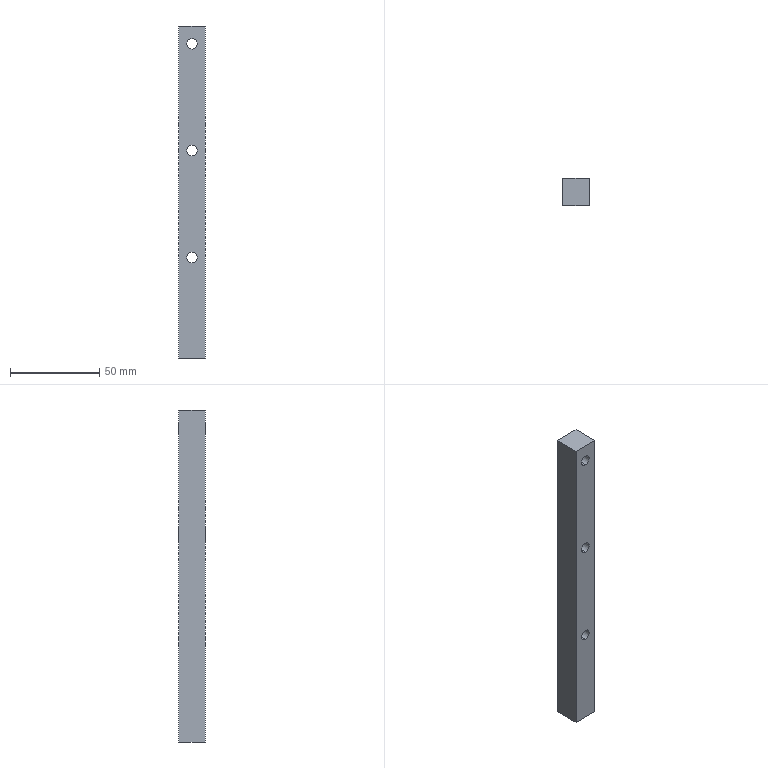Part | 1 solid | 16 faces | box 15 x 15 x 186.5 mm | volume 40084 mm3 | cylinder 8 | plane 6 | cone 2 | commonest cylinder face diameters 6 x6 6.8 x2
STEP:
#1=CARTESIAN_POINT('',(10.9,7.5,89.5));
#2=VERTEX_POINT('',#1);
#3=CARTESIAN_POINT('',(4.1,7.5,89.5));
#4=VERTEX_POINT('',#3);
#5=CARTESIAN_POINT('',(7.5,7.5,89.5));
#6=DIRECTION('',(0.,0.,-1.));
#7=DIRECTION('',(-1.,0.,0.));
#8=AXIS2_PLACEMENT_3D('',#5,#6,#7);
#9=CIRCLE('',#8,3.4);
#10=EDGE_CURVE('',#2,#4,#9,.T.);
#11=ORIENTED_EDGE('',*,*,#10,.F.);
#12=CARTESIAN_POINT('',(10.9,7.5,73.5));
#13=VERTEX_POINT('',#12);
#14=CARTESIAN_POINT('',(10.9,7.5,73.5));
#15=DIRECTION('',(0.,0.,-1.));
#16=VECTOR('',#15,1000.);
#17=LINE('',#14,#16);
#18=EDGE_CURVE('',#2,#13,#17,.T.);
#19=ORIENTED_EDGE('',*,*,#18,.T.);
#20=CARTESIAN_POINT('',(4.1,7.5,73.5));
#21=VERTEX_POINT('',#20);
#22=CARTESIAN_POINT('',(7.5,7.5,73.5));
#23=DIRECTION('',(0.,0.,-1.));
#24=DIRECTION('',(-1.,0.,0.));
#25=AXIS2_PLACEMENT_3D('',#22,#23,#24);
#26=CIRCLE('',#25,3.4);
#27=EDGE_CURVE('',#13,#21,#26,.T.);
#28=ORIENTED_EDGE('',*,*,#27,.T.);
#29=CARTESIAN_POINT('',(4.1,7.5,73.5));
#30=DIRECTION('',(0.,0.,-1.));
#31=VECTOR('',#30,1000.);
#32=LINE('',#29,#31);
#33=EDGE_CURVE('',#4,#21,#32,.T.);
#34=ORIENTED_EDGE('',*,*,#33,.F.);
#35=EDGE_LOOP('',(#11,#19,#28,#34));
#36=FACE_OUTER_BOUND('',#35,.T.);
#37=CARTESIAN_POINT('',(7.5,7.5,73.5));
#38=DIRECTION('',(0.,0.,-1.));
#39=DIRECTION('',(-1.,0.,0.));
#40=AXIS2_PLACEMENT_3D('',#37,#38,#39);
#41=CYLINDRICAL_SURFACE('',#40,3.4);
#42=ADVANCED_FACE('',(#36),#41,.F.);
#43=CARTESIAN_POINT('',(7.5,7.5,91.543));
#44=VERTEX_POINT('',#43);
#45=CARTESIAN_POINT('',(4.1,7.5,89.5));
#46=DIRECTION('',(-0.8572,0.,-0.515));
#47=VECTOR('',#46,1000.);
#48=LINE('',#45,#47);
#49=EDGE_CURVE('',#44,#4,#48,.T.);
#50=ORIENTED_EDGE('',*,*,#49,.F.);
#51=CARTESIAN_POINT('',(10.9,7.5,89.5));
#52=DIRECTION('',(0.8572,0.,-0.515));
#53=VECTOR('',#52,1000.);
#54=LINE('',#51,#53);
#55=EDGE_CURVE('',#44,#2,#54,.T.);
#56=ORIENTED_EDGE('',*,*,#55,.T.);
#57=ORIENTED_EDGE('',*,*,#10,.T.);
#58=EDGE_LOOP('',(#50,#56,#57));
#59=FACE_OUTER_BOUND('',#58,.T.);
#60=CARTESIAN_POINT('',(7.5,7.5,89.5));
#61=DIRECTION('',(0.,0.,-1.));
#62=DIRECTION('',(-1.,0.,0.));
#63=AXIS2_PLACEMENT_3D('',#60,#61,#62);
#64=CONICAL_SURFACE('',#63,3.4,1.03);
#65=ADVANCED_FACE('',(#59),#64,.F.);
#66=CARTESIAN_POINT('',(7.5,0.,247.));
#67=VERTEX_POINT('',#66);
#68=CARTESIAN_POINT('',(7.5,0.,253.));
#69=VERTEX_POINT('',#68);
#70=CARTESIAN_POINT('',(7.5,0.,250.));
#71=DIRECTION('',(0.,1.,0.));
#72=DIRECTION('',(0.,0.,1.));
#73=AXIS2_PLACEMENT_3D('',#70,#71,#72);
#74=CIRCLE('',#73,3.);
#75=EDGE_CURVE('',#67,#69,#74,.T.);
#76=ORIENTED_EDGE('',*,*,#75,.F.);
#77=CARTESIAN_POINT('',(7.5,15.,247.));
#78=VERTEX_POINT('',#77);
#79=CARTESIAN_POINT('',(7.5,-35.,247.));
#80=DIRECTION('',(0.,1.,0.));
#81=VECTOR('',#80,1000.);
#82=LINE('',#79,#81);
#83=EDGE_CURVE('',#67,#78,#82,.T.);
#84=ORIENTED_EDGE('',*,*,#83,.T.);
#85=CARTESIAN_POINT('',(7.5,15.,253.));
#86=VERTEX_POINT('',#85);
#87=CARTESIAN_POINT('',(7.5,15.,250.));
#88=DIRECTION('',(0.,1.,0.));
#89=DIRECTION('',(0.,0.,1.));
#90=AXIS2_PLACEMENT_3D('',#87,#88,#89);
#91=CIRCLE('',#90,3.);
#92=EDGE_CURVE('',#78,#86,#91,.T.);
#93=ORIENTED_EDGE('',*,*,#92,.T.);
#94=CARTESIAN_POINT('',(7.5,-35.,253.));
#95=DIRECTION('',(0.,1.,0.));
#96=VECTOR('',#95,1000.);
#97=LINE('',#94,#96);
#98=EDGE_CURVE('',#69,#86,#97,.T.);
#99=ORIENTED_EDGE('',*,*,#98,.F.);
#100=EDGE_LOOP('',(#76,#84,#93,#99));
#101=FACE_OUTER_BOUND('',#100,.T.);
#102=CARTESIAN_POINT('',(7.5,-35.,250.));
#103=DIRECTION('',(0.,1.,0.));
#104=DIRECTION('',(0.,0.,1.));
#105=AXIS2_PLACEMENT_3D('',#102,#103,#104);
#106=CYLINDRICAL_SURFACE('',#105,3.);
#107=ADVANCED_FACE('',(#101),#106,.F.);
#108=CARTESIAN_POINT('',(7.5,0.,187.));
#109=VERTEX_POINT('',#108);
#110=CARTESIAN_POINT('',(7.5,0.,193.));
#111=VERTEX_POINT('',#110);
#112=CARTESIAN_POINT('',(7.5,0.,190.));
#113=DIRECTION('',(0.,1.,0.));
#114=DIRECTION('',(0.,0.,1.));
#115=AXIS2_PLACEMENT_3D('',#112,#113,#114);
#116=CIRCLE('',#115,3.);
#117=EDGE_CURVE('',#109,#111,#116,.T.);
#118=ORIENTED_EDGE('',*,*,#117,.F.);
#119=CARTESIAN_POINT('',(7.5,15.,187.));
#120=VERTEX_POINT('',#119);
#121=CARTESIAN_POINT('',(7.5,-35.,187.));
#122=DIRECTION('',(0.,1.,0.));
#123=VECTOR('',#122,1000.);
#124=LINE('',#121,#123);
#125=EDGE_CURVE('',#109,#120,#124,.T.);
#126=ORIENTED_EDGE('',*,*,#125,.T.);
#127=CARTESIAN_POINT('',(7.5,15.,193.));
#128=VERTEX_POINT('',#127);
#129=CARTESIAN_POINT('',(7.5,15.,190.));
#130=DIRECTION('',(0.,1.,0.));
#131=DIRECTION('',(0.,0.,1.));
#132=AXIS2_PLACEMENT_3D('',#129,#130,#131);
#133=CIRCLE('',#132,3.);
#134=EDGE_CURVE('',#120,#128,#133,.T.);
#135=ORIENTED_EDGE('',*,*,#134,.T.);
#136=CARTESIAN_POINT('',(7.5,-35.,193.));
#137=DIRECTION('',(0.,1.,0.));
#138=VECTOR('',#137,1000.);
#139=LINE('',#136,#138);
#140=EDGE_CURVE('',#111,#128,#139,.T.);
#141=ORIENTED_EDGE('',*,*,#140,.F.);
#142=EDGE_LOOP('',(#118,#126,#135,#141));
#143=FACE_OUTER_BOUND('',#142,.T.);
#144=CARTESIAN_POINT('',(7.5,-35.,190.));
#145=DIRECTION('',(0.,1.,0.));
#146=DIRECTION('',(0.,0.,1.));
#147=AXIS2_PLACEMENT_3D('',#144,#145,#146);
#148=CYLINDRICAL_SURFACE('',#147,3.);
#149=ADVANCED_FACE('',(#143),#148,.F.);
#150=CARTESIAN_POINT('',(7.5,0.,127.));
#151=VERTEX_POINT('',#150);
#152=CARTESIAN_POINT('',(7.5,0.,133.));
#153=VERTEX_POINT('',#152);
#154=CARTESIAN_POINT('',(7.5,0.,130.));
#155=DIRECTION('',(0.,1.,0.));
#156=DIRECTION('',(0.,0.,1.));
#157=AXIS2_PLACEMENT_3D('',#154,#155,#156);
#158=CIRCLE('',#157,3.);
#159=EDGE_CURVE('',#151,#153,#158,.T.);
#160=ORIENTED_EDGE('',*,*,#159,.F.);
#161=CARTESIAN_POINT('',(7.5,15.,127.));
#162=VERTEX_POINT('',#161);
#163=CARTESIAN_POINT('',(7.5,-35.,127.));
#164=DIRECTION('',(0.,1.,0.));
#165=VECTOR('',#164,1000.);
#166=LINE('',#163,#165);
#167=EDGE_CURVE('',#151,#162,#166,.T.);
#168=ORIENTED_EDGE('',*,*,#167,.T.);
#169=CARTESIAN_POINT('',(7.5,15.,133.));
#170=VERTEX_POINT('',#169);
#171=CARTESIAN_POINT('',(7.5,15.,130.));
#172=DIRECTION('',(0.,1.,0.));
#173=DIRECTION('',(0.,0.,1.));
#174=AXIS2_PLACEMENT_3D('',#171,#172,#173);
#175=CIRCLE('',#174,3.);
#176=EDGE_CURVE('',#162,#170,#175,.T.);
#177=ORIENTED_EDGE('',*,*,#176,.T.);
#178=CARTESIAN_POINT('',(7.5,-35.,133.));
#179=DIRECTION('',(0.,1.,0.));
#180=VECTOR('',#179,1000.);
#181=LINE('',#178,#180);
#182=EDGE_CURVE('',#153,#170,#181,.T.);
#183=ORIENTED_EDGE('',*,*,#182,.F.);
#184=EDGE_LOOP('',(#160,#168,#177,#183));
#185=FACE_OUTER_BOUND('',#184,.T.);
#186=CARTESIAN_POINT('',(7.5,-35.,130.));
#187=DIRECTION('',(0.,1.,0.));
#188=DIRECTION('',(0.,0.,1.));
#189=AXIS2_PLACEMENT_3D('',#186,#187,#188);
#190=CYLINDRICAL_SURFACE('',#189,3.);
#191=ADVANCED_FACE('',(#185),#190,.F.);
#192=CARTESIAN_POINT('',(0.,0.,73.5));
#193=VERTEX_POINT('',#192);
#194=CARTESIAN_POINT('',(0.,15.,73.5));
#195=VERTEX_POINT('',#194);
#196=CARTESIAN_POINT('',(0.,0.,73.5));
#197=DIRECTION('',(0.,1.,0.));
#198=VECTOR('',#197,1000.);
#199=LINE('',#196,#198);
#200=EDGE_CURVE('',#193,#195,#199,.T.);
#201=ORIENTED_EDGE('',*,*,#200,.F.);
#202=CARTESIAN_POINT('',(0.,0.,260.));
#203=VERTEX_POINT('',#202);
#204=CARTESIAN_POINT('',(0.,0.,700.));
#205=DIRECTION('',(0.,0.,-1.));
#206=VECTOR('',#205,1000.);
#207=LINE('',#204,#206);
#208=EDGE_CURVE('',#203,#193,#207,.T.);
#209=ORIENTED_EDGE('',*,*,#208,.F.);
#210=CARTESIAN_POINT('',(0.,15.,260.));
#211=VERTEX_POINT('',#210);
#212=CARTESIAN_POINT('',(0.,15.,260.));
#213=DIRECTION('',(0.,-1.,0.));
#214=VECTOR('',#213,1000.);
#215=LINE('',#212,#214);
#216=EDGE_CURVE('',#211,#203,#215,.T.);
#217=ORIENTED_EDGE('',*,*,#216,.F.);
#218=CARTESIAN_POINT('',(0.,15.,700.));
#219=DIRECTION('',(0.,0.,-1.));
#220=VECTOR('',#219,1000.);
#221=LINE('',#218,#220);
#222=EDGE_CURVE('',#211,#195,#221,.T.);
#223=ORIENTED_EDGE('',*,*,#222,.T.);
#224=EDGE_LOOP('',(#201,#209,#217,#223));
#225=FACE_OUTER_BOUND('',#224,.T.);
#226=CARTESIAN_POINT('',(0.,0.,700.));
#227=DIRECTION('',(1.,0.,0.));
#228=DIRECTION('',(0.,0.,-1.));
#229=AXIS2_PLACEMENT_3D('',#226,#227,#228);
#230=PLANE('',#229);
#231=ADVANCED_FACE('',(#225),#230,.F.);
#232=CARTESIAN_POINT('',(7.5,0.,130.));
#233=DIRECTION('',(0.,1.,0.));
#234=DIRECTION('',(0.,0.,1.));
#235=AXIS2_PLACEMENT_3D('',#232,#233,#234);
#236=CIRCLE('',#235,3.);
#237=EDGE_CURVE('',#153,#151,#236,.T.);
#238=ORIENTED_EDGE('',*,*,#237,.T.);
#239=ORIENTED_EDGE('',*,*,#159,.T.);
#240=EDGE_LOOP('',(#238,#239));
#241=FACE_BOUND('',#240,.T.);
#242=CARTESIAN_POINT('',(7.5,0.,190.));
#243=DIRECTION('',(0.,1.,0.));
#244=DIRECTION('',(0.,0.,1.));
#245=AXIS2_PLACEMENT_3D('',#242,#243,#244);
#246=CIRCLE('',#245,3.);
#247=EDGE_CURVE('',#111,#109,#246,.T.);
#248=ORIENTED_EDGE('',*,*,#247,.T.);
#249=ORIENTED_EDGE('',*,*,#117,.T.);
#250=EDGE_LOOP('',(#248,#249));
#251=FACE_BOUND('',#250,.T.);
#252=CARTESIAN_POINT('',(7.5,0.,250.));
#253=DIRECTION('',(0.,1.,0.));
#254=DIRECTION('',(0.,0.,1.));
#255=AXIS2_PLACEMENT_3D('',#252,#253,#254);
#256=CIRCLE('',#255,3.);
#257=EDGE_CURVE('',#69,#67,#256,.T.);
#258=ORIENTED_EDGE('',*,*,#257,.T.);
#259=ORIENTED_EDGE('',*,*,#75,.T.);
#260=EDGE_LOOP('',(#258,#259));
#261=FACE_BOUND('',#260,.T.);
#262=CARTESIAN_POINT('',(15.,0.,73.5));
#263=VERTEX_POINT('',#262);
#264=CARTESIAN_POINT('',(15.,0.,73.5));
#265=DIRECTION('',(-1.,0.,0.));
#266=VECTOR('',#265,1000.);
#267=LINE('',#264,#266);
#268=EDGE_CURVE('',#263,#193,#267,.T.);
#269=ORIENTED_EDGE('',*,*,#268,.F.);
#270=CARTESIAN_POINT('',(15.,0.,260.));
#271=VERTEX_POINT('',#270);
#272=CARTESIAN_POINT('',(15.,0.,700.));
#273=DIRECTION('',(0.,0.,-1.));
#274=VECTOR('',#273,1000.);
#275=LINE('',#272,#274);
#276=EDGE_CURVE('',#271,#263,#275,.T.);
#277=ORIENTED_EDGE('',*,*,#276,.F.);
#278=CARTESIAN_POINT('',(0.,0.,260.));
#279=DIRECTION('',(1.,0.,0.));
#280=VECTOR('',#279,1000.);
#281=LINE('',#278,#280);
#282=EDGE_CURVE('',#203,#271,#281,.T.);
#283=ORIENTED_EDGE('',*,*,#282,.F.);
#284=ORIENTED_EDGE('',*,*,#208,.T.);
#285=EDGE_LOOP('',(#269,#277,#283,#284));
#286=FACE_OUTER_BOUND('',#285,.T.);
#287=CARTESIAN_POINT('',(0.,0.,700.));
#288=DIRECTION('',(0.,1.,0.));
#289=DIRECTION('',(0.,0.,1.));
#290=AXIS2_PLACEMENT_3D('',#287,#288,#289);
#291=PLANE('',#290);
#292=ADVANCED_FACE('',(#241,#251,#261,#286),#291,.F.);
#293=CARTESIAN_POINT('',(15.,15.,73.5));
#294=VERTEX_POINT('',#293);
#295=CARTESIAN_POINT('',(15.,15.,73.5));
#296=DIRECTION('',(0.,-1.,0.));
#297=VECTOR('',#296,1000.);
#298=LINE('',#295,#297);
#299=EDGE_CURVE('',#294,#263,#298,.T.);
#300=ORIENTED_EDGE('',*,*,#299,.F.);
#301=CARTESIAN_POINT('',(15.,15.,260.));
#302=VERTEX_POINT('',#301);
#303=CARTESIAN_POINT('',(15.,15.,700.));
#304=DIRECTION('',(0.,0.,-1.));
#305=VECTOR('',#304,1000.);
#306=LINE('',#303,#305);
#307=EDGE_CURVE('',#302,#294,#306,.T.);
#308=ORIENTED_EDGE('',*,*,#307,.F.);
#309=CARTESIAN_POINT('',(15.,0.,260.));
#310=DIRECTION('',(0.,1.,0.));
#311=VECTOR('',#310,1000.);
#312=LINE('',#309,#311);
#313=EDGE_CURVE('',#271,#302,#312,.T.);
#314=ORIENTED_EDGE('',*,*,#313,.F.);
#315=ORIENTED_EDGE('',*,*,#276,.T.);
#316=EDGE_LOOP('',(#300,#308,#314,#315));
#317=FACE_OUTER_BOUND('',#316,.T.);
#318=CARTESIAN_POINT('',(15.,0.,700.));
#319=DIRECTION('',(-1.,0.,0.));
#320=DIRECTION('',(0.,0.,1.));
#321=AXIS2_PLACEMENT_3D('',#318,#319,#320);
#322=PLANE('',#321);
#323=ADVANCED_FACE('',(#317),#322,.F.);
#324=CARTESIAN_POINT('',(7.5,15.,130.));
#325=DIRECTION('',(0.,1.,0.));
#326=DIRECTION('',(0.,0.,1.));
#327=AXIS2_PLACEMENT_3D('',#324,#325,#326);
#328=CIRCLE('',#327,3.);
#329=EDGE_CURVE('',#170,#162,#328,.T.);
#330=ORIENTED_EDGE('',*,*,#329,.F.);
#331=ORIENTED_EDGE('',*,*,#176,.F.);
#332=EDGE_LOOP('',(#330,#331));
#333=FACE_BOUND('',#332,.T.);
#334=CARTESIAN_POINT('',(7.5,15.,190.));
#335=DIRECTION('',(0.,1.,0.));
#336=DIRECTION('',(0.,0.,1.));
#337=AXIS2_PLACEMENT_3D('',#334,#335,#336);
#338=CIRCLE('',#337,3.);
#339=EDGE_CURVE('',#128,#120,#338,.T.);
#340=ORIENTED_EDGE('',*,*,#339,.F.);
#341=ORIENTED_EDGE('',*,*,#134,.F.);
#342=EDGE_LOOP('',(#340,#341));
#343=FACE_BOUND('',#342,.T.);
#344=CARTESIAN_POINT('',(7.5,15.,250.));
#345=DIRECTION('',(0.,1.,0.));
#346=DIRECTION('',(0.,0.,1.));
#347=AXIS2_PLACEMENT_3D('',#344,#345,#346);
#348=CIRCLE('',#347,3.);
#349=EDGE_CURVE('',#86,#78,#348,.T.);
#350=ORIENTED_EDGE('',*,*,#349,.F.);
#351=ORIENTED_EDGE('',*,*,#92,.F.);
#352=EDGE_LOOP('',(#350,#351));
#353=FACE_BOUND('',#352,.T.);
#354=CARTESIAN_POINT('',(0.,15.,73.5));
#355=DIRECTION('',(1.,0.,0.));
#356=VECTOR('',#355,1000.);
#357=LINE('',#354,#356);
#358=EDGE_CURVE('',#195,#294,#357,.T.);
#359=ORIENTED_EDGE('',*,*,#358,.F.);
#360=ORIENTED_EDGE('',*,*,#222,.F.);
#361=CARTESIAN_POINT('',(15.,15.,260.));
#362=DIRECTION('',(-1.,0.,0.));
#363=VECTOR('',#362,1000.);
#364=LINE('',#361,#363);
#365=EDGE_CURVE('',#302,#211,#364,.T.);
#366=ORIENTED_EDGE('',*,*,#365,.F.);
#367=ORIENTED_EDGE('',*,*,#307,.T.);
#368=EDGE_LOOP('',(#359,#360,#366,#367));
#369=FACE_OUTER_BOUND('',#368,.T.);
#370=CARTESIAN_POINT('',(0.,15.,700.));
#371=DIRECTION('',(0.,-1.,0.));
#372=DIRECTION('',(0.,0.,-1.));
#373=AXIS2_PLACEMENT_3D('',#370,#371,#372);
#374=PLANE('',#373);
#375=ADVANCED_FACE('',(#333,#343,#353,#369),#374,.F.);
#376=ORIENTED_EDGE('',*,*,#167,.F.);
#377=ORIENTED_EDGE('',*,*,#237,.F.);
#378=ORIENTED_EDGE('',*,*,#182,.T.);
#379=ORIENTED_EDGE('',*,*,#329,.T.);
#380=EDGE_LOOP('',(#376,#377,#378,#379));
#381=FACE_OUTER_BOUND('',#380,.T.);
#382=CARTESIAN_POINT('',(7.5,-35.,130.));
#383=DIRECTION('',(0.,1.,0.));
#384=DIRECTION('',(0.,0.,1.));
#385=AXIS2_PLACEMENT_3D('',#382,#383,#384);
#386=CYLINDRICAL_SURFACE('',#385,3.);
#387=ADVANCED_FACE('',(#381),#386,.F.);
#388=ORIENTED_EDGE('',*,*,#125,.F.);
#389=ORIENTED_EDGE('',*,*,#247,.F.);
#390=ORIENTED_EDGE('',*,*,#140,.T.);
#391=ORIENTED_EDGE('',*,*,#339,.T.);
#392=EDGE_LOOP('',(#388,#389,#390,#391));
#393=FACE_OUTER_BOUND('',#392,.T.);
#394=CARTESIAN_POINT('',(7.5,-35.,190.));
#395=DIRECTION('',(0.,1.,0.));
#396=DIRECTION('',(0.,0.,1.));
#397=AXIS2_PLACEMENT_3D('',#394,#395,#396);
#398=CYLINDRICAL_SURFACE('',#397,3.);
#399=ADVANCED_FACE('',(#393),#398,.F.);
#400=ORIENTED_EDGE('',*,*,#83,.F.);
#401=ORIENTED_EDGE('',*,*,#257,.F.);
#402=ORIENTED_EDGE('',*,*,#98,.T.);
#403=ORIENTED_EDGE('',*,*,#349,.T.);
#404=EDGE_LOOP('',(#400,#401,#402,#403));
#405=FACE_OUTER_BOUND('',#404,.T.);
#406=CARTESIAN_POINT('',(7.5,-35.,250.));
#407=DIRECTION('',(0.,1.,0.));
#408=DIRECTION('',(0.,0.,1.));
#409=AXIS2_PLACEMENT_3D('',#406,#407,#408);
#410=CYLINDRICAL_SURFACE('',#409,3.);
#411=ADVANCED_FACE('',(#405),#410,.F.);
#412=ORIENTED_EDGE('',*,*,#365,.T.);
#413=ORIENTED_EDGE('',*,*,#216,.T.);
#414=ORIENTED_EDGE('',*,*,#282,.T.);
#415=ORIENTED_EDGE('',*,*,#313,.T.);
#416=EDGE_LOOP('',(#412,#413,#414,#415));
#417=FACE_OUTER_BOUND('',#416,.T.);
#418=CARTESIAN_POINT('',(0.,0.,260.));
#419=DIRECTION('',(0.,0.,1.));
#420=DIRECTION('',(1.,0.,0.));
#421=AXIS2_PLACEMENT_3D('',#418,#419,#420);
#422=PLANE('',#421);
#423=ADVANCED_FACE('',(#417),#422,.T.);
#424=CARTESIAN_POINT('',(7.5,7.5,73.5));
#425=DIRECTION('',(0.,0.,-1.));
#426=DIRECTION('',(-1.,0.,0.));
#427=AXIS2_PLACEMENT_3D('',#424,#425,#426);
#428=CIRCLE('',#427,3.4);
#429=EDGE_CURVE('',#21,#13,#428,.T.);
#430=ORIENTED_EDGE('',*,*,#429,.F.);
#431=ORIENTED_EDGE('',*,*,#27,.F.);
#432=EDGE_LOOP('',(#430,#431));
#433=FACE_BOUND('',#432,.T.);
#434=ORIENTED_EDGE('',*,*,#268,.T.);
#435=ORIENTED_EDGE('',*,*,#200,.T.);
#436=ORIENTED_EDGE('',*,*,#358,.T.);
#437=ORIENTED_EDGE('',*,*,#299,.T.);
#438=EDGE_LOOP('',(#434,#435,#436,#437));
#439=FACE_OUTER_BOUND('',#438,.T.);
#440=CARTESIAN_POINT('',(0.,0.,73.5));
#441=DIRECTION('',(0.,0.,-1.));
#442=DIRECTION('',(-1.,0.,0.));
#443=AXIS2_PLACEMENT_3D('',#440,#441,#442);
#444=PLANE('',#443);
#445=ADVANCED_FACE('',(#433,#439),#444,.T.);
#446=ORIENTED_EDGE('',*,*,#55,.F.);
#447=ORIENTED_EDGE('',*,*,#49,.T.);
#448=CARTESIAN_POINT('',(7.5,7.5,89.5));
#449=DIRECTION('',(0.,0.,-1.));
#450=DIRECTION('',(-1.,0.,0.));
#451=AXIS2_PLACEMENT_3D('',#448,#449,#450);
#452=CIRCLE('',#451,3.4);
#453=EDGE_CURVE('',#4,#2,#452,.T.);
#454=ORIENTED_EDGE('',*,*,#453,.T.);
#455=EDGE_LOOP('',(#446,#447,#454));
#456=FACE_OUTER_BOUND('',#455,.T.);
#457=CARTESIAN_POINT('',(7.5,7.5,89.5));
#458=DIRECTION('',(0.,0.,-1.));
#459=DIRECTION('',(-1.,0.,0.));
#460=AXIS2_PLACEMENT_3D('',#457,#458,#459);
#461=CONICAL_SURFACE('',#460,3.4,1.03);
#462=ADVANCED_FACE('',(#456),#461,.F.);
#463=ORIENTED_EDGE('',*,*,#18,.F.);
#464=ORIENTED_EDGE('',*,*,#453,.F.);
#465=ORIENTED_EDGE('',*,*,#33,.T.);
#466=ORIENTED_EDGE('',*,*,#429,.T.);
#467=EDGE_LOOP('',(#463,#464,#465,#466));
#468=FACE_OUTER_BOUND('',#467,.T.);
#469=CARTESIAN_POINT('',(7.5,7.5,73.5));
#470=DIRECTION('',(0.,0.,-1.));
#471=DIRECTION('',(-1.,0.,0.));
#472=AXIS2_PLACEMENT_3D('',#469,#470,#471);
#473=CYLINDRICAL_SURFACE('',#472,3.4);
#474=ADVANCED_FACE('',(#468),#473,.F.);
#475=CLOSED_SHELL('',(#42,#65,#107,#149,#191,#231,#292,#323,#375,#387,#399,#411,#423,#445,#462,#474));
#476=MANIFOLD_SOLID_BREP('',#475);
#477=CARTESIAN_POINT('',(0.,0.,0.));
#478=DIRECTION('',(0.,0.,1.));
#479=DIRECTION('',(1.,0.,0.));
#480=AXIS2_PLACEMENT_3D('',#477,#478,#479);
#481=(LENGTH_UNIT()NAMED_UNIT(*)SI_UNIT(.MILLI.,.METRE.));
#482=UNCERTAINTY_MEASURE_WITH_UNIT(LENGTH_MEASURE(0.00001),#481,'','');
#483=(NAMED_UNIT(*)PLANE_ANGLE_UNIT()SI_UNIT($,.RADIAN.));
#484=(NAMED_UNIT(*)SI_UNIT($,.STERADIAN.)SOLID_ANGLE_UNIT());
#485=(GEOMETRIC_REPRESENTATION_CONTEXT(3)GLOBAL_UNCERTAINTY_ASSIGNED_CONTEXT((#482))GLOBAL_UNIT_ASSIGNED_CONTEXT((#481,#483,#484))REPRESENTATION_CONTEXT('',''));
#486=ADVANCED_BREP_SHAPE_REPRESENTATION('',(#476,#480),#485);